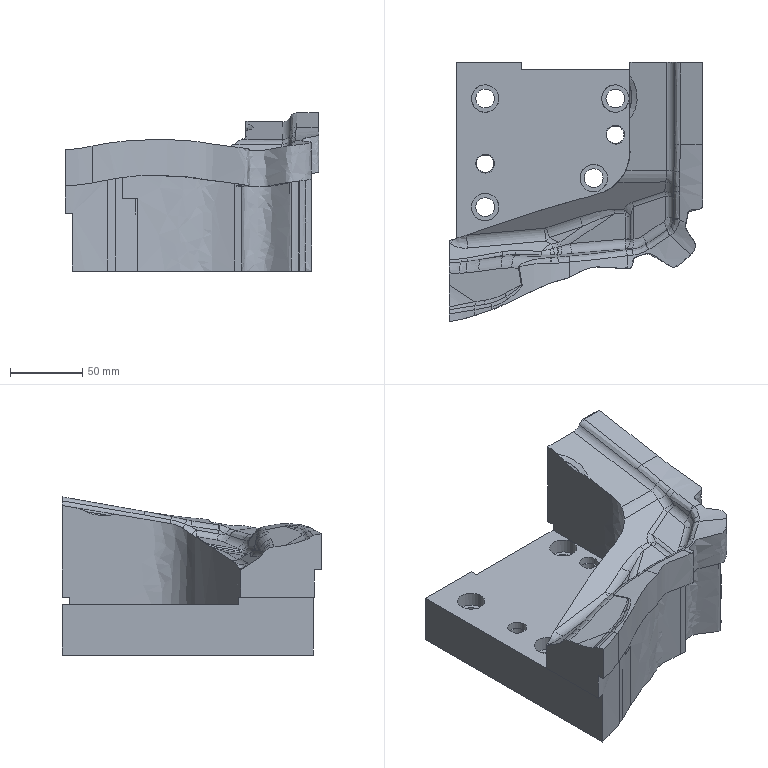Part | NX | features solid 2 | 1 solid | 164 faces | box 175.549 x 179.36 x 109.341 mm | volume 1399347 mm3 | spline 86 | cylinder 42 | plane 36 | commonest cylinder face diameters 12 x10 13 x6 16 x6 20 x5 10 x4 19 x4